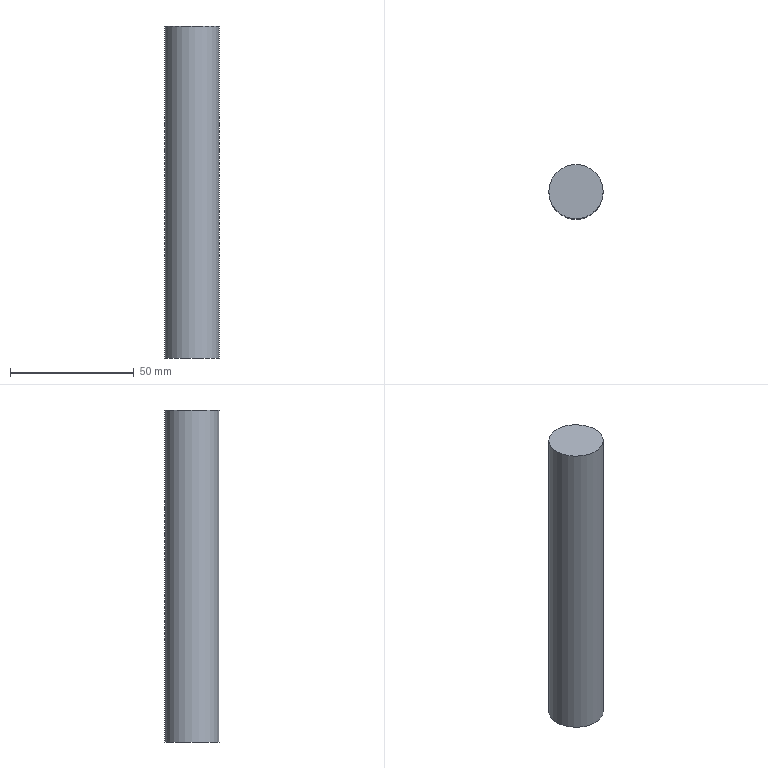Part | STEP file | solid 109 | 1 solid | 3 faces | box 22 x 22 x 134.177 mm | volume 51005 mm3 | plane 2 | cylinder 1 | commonest cylinder face diameters 22 x1